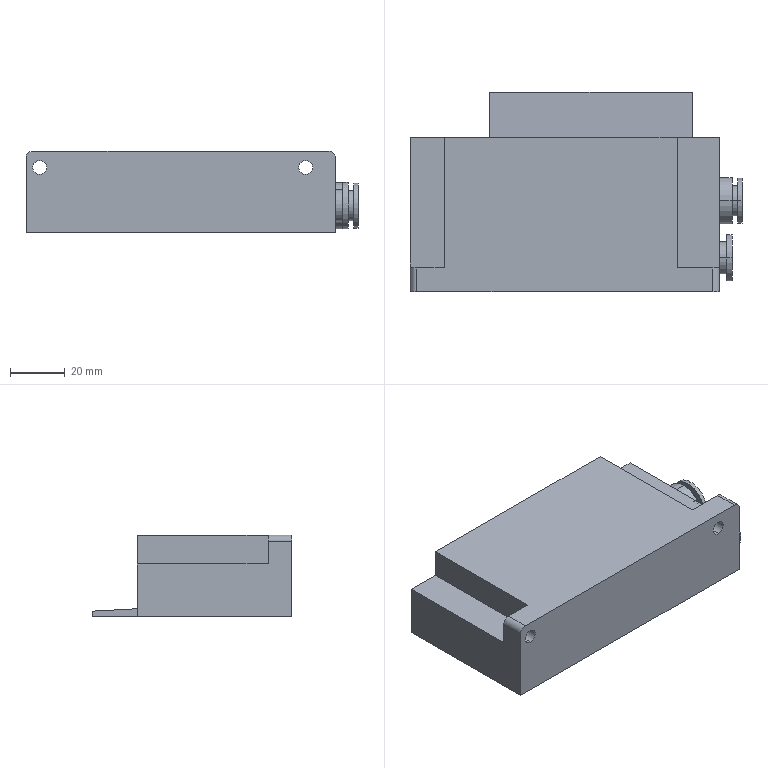Part | SolidWorks | features BaseBody 1 | 1 solid | 176 faces | box 121.7 x 73.2 x 30 mm | volume 182258 mm3 | plane 135 | cylinder 41 | commonest cylinder face diameters 5.1 x4 17 x4 1.085 x2 1.167 x2 1.316 x2 1.395 x2